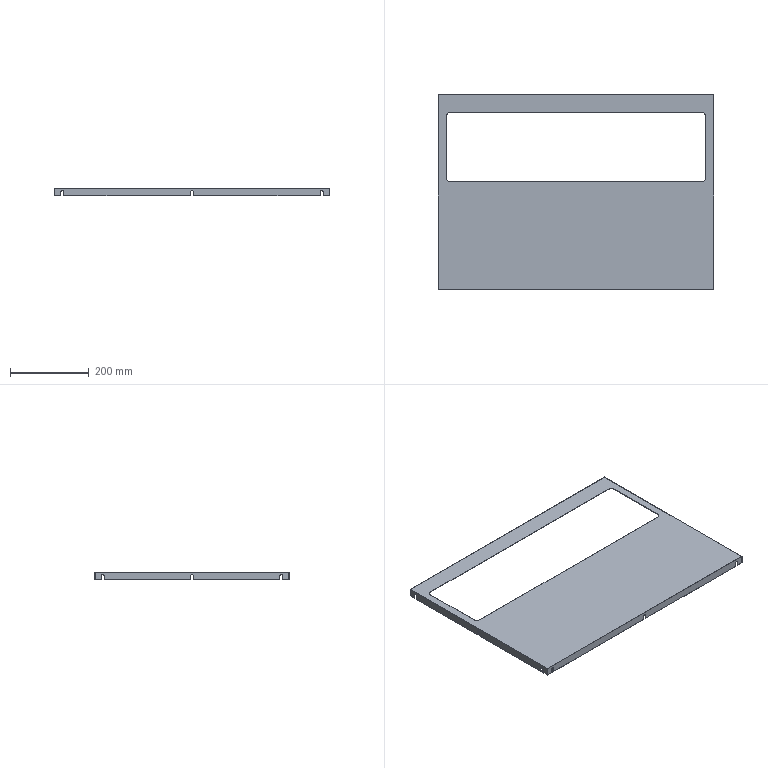Part | STEP file | PN_0006 | 1 solid | 72 faces | box 698 x 493 x 20 mm | volume 273161 mm3 | plane 50 | cylinder 22 | commonest cylinder face diameters 7 x18 20 x4